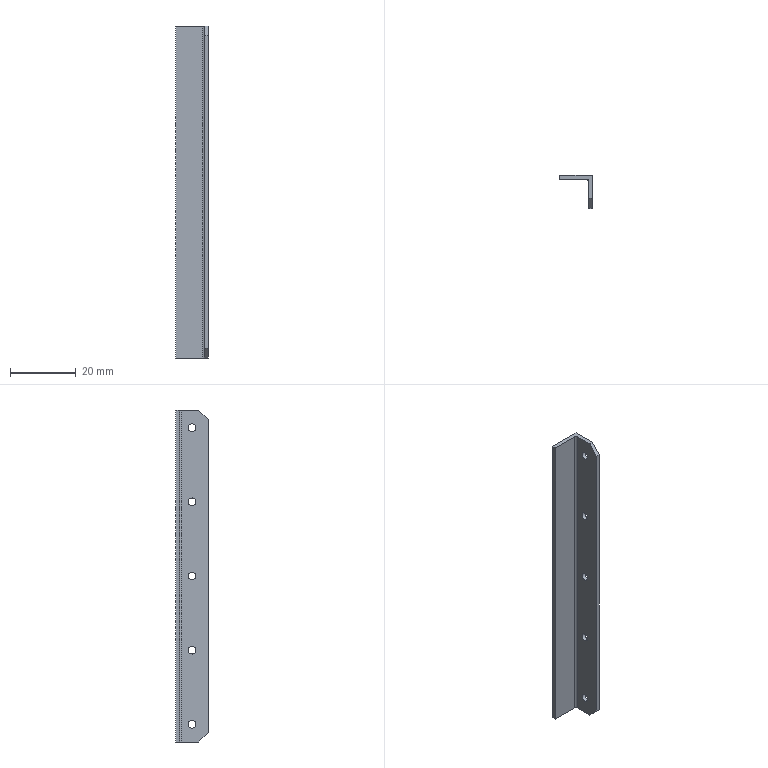Part | SolidWorks | features BaseBody 1 | 1 solid | 21 faces | box 10 x 10 x 100.8 mm | volume 2242 mm3 | cylinder 11 | plane 10 | commonest cylinder face diameters 2.4 x10 1 x1
STEP:
#1=CARTESIAN_POINT('',(-1.2,-5.,-74.1));
#2=VERTEX_POINT('',#1);
#3=CARTESIAN_POINT('',(-1.2,-5.,-71.7));
#4=VERTEX_POINT('',#3);
#5=CARTESIAN_POINT('',(-1.2,-5.,-72.9));
#6=DIRECTION('',(-1.,0.,0.));
#7=DIRECTION('',(0.,0.,-1.));
#8=AXIS2_PLACEMENT_3D('',#5,#6,#7);
#9=CIRCLE('',#8,1.2);
#10=EDGE_CURVE('',#2,#4,#9,.T.);
#11=ORIENTED_EDGE('',*,*,#10,.T.);
#12=CARTESIAN_POINT('',(0.,-5.,-71.7));
#13=VERTEX_POINT('',#12);
#14=CARTESIAN_POINT('',(-1.2,-5.,-71.7));
#15=DIRECTION('',(1.,0.,0.));
#16=VECTOR('',#15,1000.);
#17=LINE('',#14,#16);
#18=EDGE_CURVE('',#4,#13,#17,.T.);
#19=ORIENTED_EDGE('',*,*,#18,.T.);
#20=CARTESIAN_POINT('',(0.,-5.,-74.1));
#21=VERTEX_POINT('',#20);
#22=CARTESIAN_POINT('',(0.,-5.,-72.9));
#23=DIRECTION('',(1.,0.,0.));
#24=DIRECTION('',(0.,0.,-1.));
#25=AXIS2_PLACEMENT_3D('',#22,#23,#24);
#26=CIRCLE('',#25,1.2);
#27=EDGE_CURVE('',#13,#21,#26,.T.);
#28=ORIENTED_EDGE('',*,*,#27,.T.);
#29=CARTESIAN_POINT('',(-1.2,-5.,-74.1));
#30=DIRECTION('',(1.,0.,0.));
#31=VECTOR('',#30,1000.);
#32=LINE('',#29,#31);
#33=EDGE_CURVE('',#2,#21,#32,.T.);
#34=ORIENTED_EDGE('',*,*,#33,.F.);
#35=EDGE_LOOP('',(#11,#19,#28,#34));
#36=FACE_OUTER_BOUND('',#35,.T.);
#37=CARTESIAN_POINT('',(-1.2,-5.,-72.9));
#38=DIRECTION('',(1.,0.,0.));
#39=DIRECTION('',(0.,0.,-1.));
#40=AXIS2_PLACEMENT_3D('',#37,#38,#39);
#41=CYLINDRICAL_SURFACE('',#40,1.2);
#42=ADVANCED_FACE('',(#36),#41,.F.);
#43=CARTESIAN_POINT('',(-1.2,-5.,-96.6));
#44=VERTEX_POINT('',#43);
#45=CARTESIAN_POINT('',(-1.2,-5.,-94.2));
#46=VERTEX_POINT('',#45);
#47=CARTESIAN_POINT('',(-1.2,-5.,-95.4));
#48=DIRECTION('',(-1.,0.,0.));
#49=DIRECTION('',(0.,0.,-1.));
#50=AXIS2_PLACEMENT_3D('',#47,#48,#49);
#51=CIRCLE('',#50,1.2);
#52=EDGE_CURVE('',#44,#46,#51,.T.);
#53=ORIENTED_EDGE('',*,*,#52,.T.);
#54=CARTESIAN_POINT('',(0.,-5.,-94.2));
#55=VERTEX_POINT('',#54);
#56=CARTESIAN_POINT('',(-1.2,-5.,-94.2));
#57=DIRECTION('',(1.,0.,0.));
#58=VECTOR('',#57,1000.);
#59=LINE('',#56,#58);
#60=EDGE_CURVE('',#46,#55,#59,.T.);
#61=ORIENTED_EDGE('',*,*,#60,.T.);
#62=CARTESIAN_POINT('',(0.,-5.,-96.6));
#63=VERTEX_POINT('',#62);
#64=CARTESIAN_POINT('',(0.,-5.,-95.4));
#65=DIRECTION('',(1.,0.,0.));
#66=DIRECTION('',(0.,0.,-1.));
#67=AXIS2_PLACEMENT_3D('',#64,#65,#66);
#68=CIRCLE('',#67,1.2);
#69=EDGE_CURVE('',#55,#63,#68,.T.);
#70=ORIENTED_EDGE('',*,*,#69,.T.);
#71=CARTESIAN_POINT('',(-1.2,-5.,-96.6));
#72=DIRECTION('',(1.,0.,0.));
#73=VECTOR('',#72,1000.);
#74=LINE('',#71,#73);
#75=EDGE_CURVE('',#44,#63,#74,.T.);
#76=ORIENTED_EDGE('',*,*,#75,.F.);
#77=EDGE_LOOP('',(#53,#61,#70,#76));
#78=FACE_OUTER_BOUND('',#77,.T.);
#79=CARTESIAN_POINT('',(-1.2,-5.,-95.4));
#80=DIRECTION('',(1.,0.,0.));
#81=DIRECTION('',(0.,0.,-1.));
#82=AXIS2_PLACEMENT_3D('',#79,#80,#81);
#83=CYLINDRICAL_SURFACE('',#82,1.2);
#84=ADVANCED_FACE('',(#78),#83,.F.);
#85=CARTESIAN_POINT('',(-1.2,-5.,-6.6));
#86=VERTEX_POINT('',#85);
#87=CARTESIAN_POINT('',(-1.2,-5.,-4.2));
#88=VERTEX_POINT('',#87);
#89=CARTESIAN_POINT('',(-1.2,-5.,-5.4));
#90=DIRECTION('',(-1.,0.,0.));
#91=DIRECTION('',(0.,0.,-1.));
#92=AXIS2_PLACEMENT_3D('',#89,#90,#91);
#93=CIRCLE('',#92,1.2);
#94=EDGE_CURVE('',#86,#88,#93,.T.);
#95=ORIENTED_EDGE('',*,*,#94,.T.);
#96=CARTESIAN_POINT('',(0.,-5.,-4.2));
#97=VERTEX_POINT('',#96);
#98=CARTESIAN_POINT('',(-1.2,-5.,-4.2));
#99=DIRECTION('',(1.,0.,0.));
#100=VECTOR('',#99,1000.);
#101=LINE('',#98,#100);
#102=EDGE_CURVE('',#88,#97,#101,.T.);
#103=ORIENTED_EDGE('',*,*,#102,.T.);
#104=CARTESIAN_POINT('',(0.,-5.,-6.6));
#105=VERTEX_POINT('',#104);
#106=CARTESIAN_POINT('',(0.,-5.,-5.4));
#107=DIRECTION('',(1.,0.,0.));
#108=DIRECTION('',(0.,0.,-1.));
#109=AXIS2_PLACEMENT_3D('',#106,#107,#108);
#110=CIRCLE('',#109,1.2);
#111=EDGE_CURVE('',#97,#105,#110,.T.);
#112=ORIENTED_EDGE('',*,*,#111,.T.);
#113=CARTESIAN_POINT('',(-1.2,-5.,-6.6));
#114=DIRECTION('',(1.,0.,0.));
#115=VECTOR('',#114,1000.);
#116=LINE('',#113,#115);
#117=EDGE_CURVE('',#86,#105,#116,.T.);
#118=ORIENTED_EDGE('',*,*,#117,.F.);
#119=EDGE_LOOP('',(#95,#103,#112,#118));
#120=FACE_OUTER_BOUND('',#119,.T.);
#121=CARTESIAN_POINT('',(-1.2,-5.,-5.4));
#122=DIRECTION('',(1.,0.,0.));
#123=DIRECTION('',(0.,0.,-1.));
#124=AXIS2_PLACEMENT_3D('',#121,#122,#123);
#125=CYLINDRICAL_SURFACE('',#124,1.2);
#126=ADVANCED_FACE('',(#120),#125,.F.);
#127=CARTESIAN_POINT('',(-1.2,-5.,-51.6));
#128=VERTEX_POINT('',#127);
#129=CARTESIAN_POINT('',(-1.2,-5.,-49.2));
#130=VERTEX_POINT('',#129);
#131=CARTESIAN_POINT('',(-1.2,-5.,-50.4));
#132=DIRECTION('',(-1.,0.,0.));
#133=DIRECTION('',(0.,0.,-1.));
#134=AXIS2_PLACEMENT_3D('',#131,#132,#133);
#135=CIRCLE('',#134,1.2);
#136=EDGE_CURVE('',#128,#130,#135,.T.);
#137=ORIENTED_EDGE('',*,*,#136,.T.);
#138=CARTESIAN_POINT('',(0.,-5.,-49.2));
#139=VERTEX_POINT('',#138);
#140=CARTESIAN_POINT('',(-1.2,-5.,-49.2));
#141=DIRECTION('',(1.,0.,0.));
#142=VECTOR('',#141,1000.);
#143=LINE('',#140,#142);
#144=EDGE_CURVE('',#130,#139,#143,.T.);
#145=ORIENTED_EDGE('',*,*,#144,.T.);
#146=CARTESIAN_POINT('',(0.,-5.,-51.6));
#147=VERTEX_POINT('',#146);
#148=CARTESIAN_POINT('',(0.,-5.,-50.4));
#149=DIRECTION('',(1.,0.,0.));
#150=DIRECTION('',(0.,0.,-1.));
#151=AXIS2_PLACEMENT_3D('',#148,#149,#150);
#152=CIRCLE('',#151,1.2);
#153=EDGE_CURVE('',#139,#147,#152,.T.);
#154=ORIENTED_EDGE('',*,*,#153,.T.);
#155=CARTESIAN_POINT('',(-1.2,-5.,-51.6));
#156=DIRECTION('',(1.,0.,0.));
#157=VECTOR('',#156,1000.);
#158=LINE('',#155,#157);
#159=EDGE_CURVE('',#128,#147,#158,.T.);
#160=ORIENTED_EDGE('',*,*,#159,.F.);
#161=EDGE_LOOP('',(#137,#145,#154,#160));
#162=FACE_OUTER_BOUND('',#161,.T.);
#163=CARTESIAN_POINT('',(-1.2,-5.,-50.4));
#164=DIRECTION('',(1.,0.,0.));
#165=DIRECTION('',(0.,0.,-1.));
#166=AXIS2_PLACEMENT_3D('',#163,#164,#165);
#167=CYLINDRICAL_SURFACE('',#166,1.2);
#168=ADVANCED_FACE('',(#162),#167,.F.);
#169=CARTESIAN_POINT('',(-1.2,-5.,-29.1));
#170=VERTEX_POINT('',#169);
#171=CARTESIAN_POINT('',(-1.2,-5.,-26.7));
#172=VERTEX_POINT('',#171);
#173=CARTESIAN_POINT('',(-1.2,-5.,-27.9));
#174=DIRECTION('',(-1.,0.,0.));
#175=DIRECTION('',(0.,0.,-1.));
#176=AXIS2_PLACEMENT_3D('',#173,#174,#175);
#177=CIRCLE('',#176,1.2);
#178=EDGE_CURVE('',#170,#172,#177,.T.);
#179=ORIENTED_EDGE('',*,*,#178,.T.);
#180=CARTESIAN_POINT('',(0.,-5.,-26.7));
#181=VERTEX_POINT('',#180);
#182=CARTESIAN_POINT('',(-1.2,-5.,-26.7));
#183=DIRECTION('',(1.,0.,0.));
#184=VECTOR('',#183,1000.);
#185=LINE('',#182,#184);
#186=EDGE_CURVE('',#172,#181,#185,.T.);
#187=ORIENTED_EDGE('',*,*,#186,.T.);
#188=CARTESIAN_POINT('',(0.,-5.,-29.1));
#189=VERTEX_POINT('',#188);
#190=CARTESIAN_POINT('',(0.,-5.,-27.9));
#191=DIRECTION('',(1.,0.,0.));
#192=DIRECTION('',(0.,0.,-1.));
#193=AXIS2_PLACEMENT_3D('',#190,#191,#192);
#194=CIRCLE('',#193,1.2);
#195=EDGE_CURVE('',#181,#189,#194,.T.);
#196=ORIENTED_EDGE('',*,*,#195,.T.);
#197=CARTESIAN_POINT('',(-1.2,-5.,-29.1));
#198=DIRECTION('',(1.,0.,0.));
#199=VECTOR('',#198,1000.);
#200=LINE('',#197,#199);
#201=EDGE_CURVE('',#170,#189,#200,.T.);
#202=ORIENTED_EDGE('',*,*,#201,.F.);
#203=EDGE_LOOP('',(#179,#187,#196,#202));
#204=FACE_OUTER_BOUND('',#203,.T.);
#205=CARTESIAN_POINT('',(-1.2,-5.,-27.9));
#206=DIRECTION('',(1.,0.,0.));
#207=DIRECTION('',(0.,0.,-1.));
#208=AXIS2_PLACEMENT_3D('',#205,#206,#207);
#209=CYLINDRICAL_SURFACE('',#208,1.2);
#210=ADVANCED_FACE('',(#204),#209,.F.);
#211=ORIENTED_EDGE('',*,*,#18,.F.);
#212=CARTESIAN_POINT('',(-1.2,-5.,-72.9));
#213=DIRECTION('',(-1.,0.,0.));
#214=DIRECTION('',(0.,0.,-1.));
#215=AXIS2_PLACEMENT_3D('',#212,#213,#214);
#216=CIRCLE('',#215,1.2);
#217=EDGE_CURVE('',#4,#2,#216,.T.);
#218=ORIENTED_EDGE('',*,*,#217,.T.);
#219=ORIENTED_EDGE('',*,*,#33,.T.);
#220=CARTESIAN_POINT('',(0.,-5.,-72.9));
#221=DIRECTION('',(1.,0.,0.));
#222=DIRECTION('',(0.,0.,-1.));
#223=AXIS2_PLACEMENT_3D('',#220,#221,#222);
#224=CIRCLE('',#223,1.2);
#225=EDGE_CURVE('',#21,#13,#224,.T.);
#226=ORIENTED_EDGE('',*,*,#225,.T.);
#227=EDGE_LOOP('',(#211,#218,#219,#226));
#228=FACE_OUTER_BOUND('',#227,.T.);
#229=CARTESIAN_POINT('',(-1.2,-5.,-72.9));
#230=DIRECTION('',(1.,0.,0.));
#231=DIRECTION('',(0.,0.,-1.));
#232=AXIS2_PLACEMENT_3D('',#229,#230,#231);
#233=CYLINDRICAL_SURFACE('',#232,1.2);
#234=ADVANCED_FACE('',(#228),#233,.F.);
#235=CARTESIAN_POINT('',(0.,-5.,-95.4));
#236=DIRECTION('',(1.,0.,0.));
#237=DIRECTION('',(0.,0.,-1.));
#238=AXIS2_PLACEMENT_3D('',#235,#236,#237);
#239=CIRCLE('',#238,1.2);
#240=EDGE_CURVE('',#63,#55,#239,.T.);
#241=ORIENTED_EDGE('',*,*,#240,.F.);
#242=ORIENTED_EDGE('',*,*,#69,.F.);
#243=EDGE_LOOP('',(#241,#242));
#244=FACE_BOUND('',#243,.T.);
#245=CARTESIAN_POINT('',(0.,-5.,-5.4));
#246=DIRECTION('',(1.,0.,0.));
#247=DIRECTION('',(0.,0.,-1.));
#248=AXIS2_PLACEMENT_3D('',#245,#246,#247);
#249=CIRCLE('',#248,1.2);
#250=EDGE_CURVE('',#105,#97,#249,.T.);
#251=ORIENTED_EDGE('',*,*,#250,.F.);
#252=ORIENTED_EDGE('',*,*,#111,.F.);
#253=EDGE_LOOP('',(#251,#252));
#254=FACE_BOUND('',#253,.T.);
#255=CARTESIAN_POINT('',(0.,-5.,-50.4));
#256=DIRECTION('',(1.,0.,0.));
#257=DIRECTION('',(0.,0.,-1.));
#258=AXIS2_PLACEMENT_3D('',#255,#256,#257);
#259=CIRCLE('',#258,1.2);
#260=EDGE_CURVE('',#147,#139,#259,.T.);
#261=ORIENTED_EDGE('',*,*,#260,.F.);
#262=ORIENTED_EDGE('',*,*,#153,.F.);
#263=EDGE_LOOP('',(#261,#262));
#264=FACE_BOUND('',#263,.T.);
#265=CARTESIAN_POINT('',(0.,-5.,-27.9));
#266=DIRECTION('',(1.,0.,0.));
#267=DIRECTION('',(0.,0.,-1.));
#268=AXIS2_PLACEMENT_3D('',#265,#266,#267);
#269=CIRCLE('',#268,1.2);
#270=EDGE_CURVE('',#189,#181,#269,.T.);
#271=ORIENTED_EDGE('',*,*,#270,.F.);
#272=ORIENTED_EDGE('',*,*,#195,.F.);
#273=EDGE_LOOP('',(#271,#272));
#274=FACE_BOUND('',#273,.T.);
#275=ORIENTED_EDGE('',*,*,#225,.F.);
#276=ORIENTED_EDGE('',*,*,#27,.F.);
#277=EDGE_LOOP('',(#275,#276));
#278=FACE_BOUND('',#277,.T.);
#279=CARTESIAN_POINT('',(0.,0.,0.));
#280=VERTEX_POINT('',#279);
#281=CARTESIAN_POINT('',(0.,0.,-100.8));
#282=VERTEX_POINT('',#281);
#283=CARTESIAN_POINT('',(0.,0.,-50.4));
#284=DIRECTION('',(0.,0.,-1.));
#285=VECTOR('',#284,1000.);
#286=LINE('',#283,#285);
#287=EDGE_CURVE('',#280,#282,#286,.T.);
#288=ORIENTED_EDGE('',*,*,#287,.F.);
#289=CARTESIAN_POINT('',(0.,-7.,0.));
#290=VERTEX_POINT('',#289);
#291=CARTESIAN_POINT('',(0.,-5.,0.));
#292=DIRECTION('',(0.,1.,0.));
#293=VECTOR('',#292,1000.);
#294=LINE('',#291,#293);
#295=EDGE_CURVE('',#290,#280,#294,.T.);
#296=ORIENTED_EDGE('',*,*,#295,.F.);
#297=CARTESIAN_POINT('',(0.,-10.,-3.));
#298=VERTEX_POINT('',#297);
#299=CARTESIAN_POINT('',(0.,-10.,-3.));
#300=DIRECTION('',(0.,0.7071,0.7071));
#301=VECTOR('',#300,1000.);
#302=LINE('',#299,#301);
#303=EDGE_CURVE('',#298,#290,#302,.T.);
#304=ORIENTED_EDGE('',*,*,#303,.F.);
#305=CARTESIAN_POINT('',(0.,-10.,-97.8));
#306=VERTEX_POINT('',#305);
#307=CARTESIAN_POINT('',(0.,-10.,-50.4));
#308=DIRECTION('',(0.,0.,1.));
#309=VECTOR('',#308,1000.);
#310=LINE('',#307,#309);
#311=EDGE_CURVE('',#306,#298,#310,.T.);
#312=ORIENTED_EDGE('',*,*,#311,.F.);
#313=CARTESIAN_POINT('',(0.,-7.,-100.8));
#314=VERTEX_POINT('',#313);
#315=CARTESIAN_POINT('',(0.,-10.,-97.8));
#316=DIRECTION('',(0.,-0.7071,0.7071));
#317=VECTOR('',#316,1000.);
#318=LINE('',#315,#317);
#319=EDGE_CURVE('',#314,#306,#318,.T.);
#320=ORIENTED_EDGE('',*,*,#319,.F.);
#321=CARTESIAN_POINT('',(0.,-5.,-100.8));
#322=DIRECTION('',(0.,-1.,0.));
#323=VECTOR('',#322,1000.);
#324=LINE('',#321,#323);
#325=EDGE_CURVE('',#282,#314,#324,.T.);
#326=ORIENTED_EDGE('',*,*,#325,.F.);
#327=EDGE_LOOP('',(#288,#296,#304,#312,#320,#326));
#328=FACE_OUTER_BOUND('',#327,.T.);
#329=CARTESIAN_POINT('',(0.,0.,-100.8));
#330=DIRECTION('',(-1.,0.,0.));
#331=DIRECTION('',(0.,-1.,0.));
#332=AXIS2_PLACEMENT_3D('',#329,#330,#331);
#333=PLANE('',#332);
#334=ADVANCED_FACE('',(#244,#254,#264,#274,#278,#328),#333,.F.);
#335=ORIENTED_EDGE('',*,*,#52,.F.);
#336=CARTESIAN_POINT('',(-1.2,-5.,-95.4));
#337=DIRECTION('',(-1.,0.,0.));
#338=DIRECTION('',(0.,0.,-1.));
#339=AXIS2_PLACEMENT_3D('',#336,#337,#338);
#340=CIRCLE('',#339,1.2);
#341=EDGE_CURVE('',#46,#44,#340,.T.);
#342=ORIENTED_EDGE('',*,*,#341,.F.);
#343=EDGE_LOOP('',(#335,#342));
#344=FACE_BOUND('',#343,.T.);
#345=ORIENTED_EDGE('',*,*,#94,.F.);
#346=CARTESIAN_POINT('',(-1.2,-5.,-5.4));
#347=DIRECTION('',(-1.,0.,0.));
#348=DIRECTION('',(0.,0.,-1.));
#349=AXIS2_PLACEMENT_3D('',#346,#347,#348);
#350=CIRCLE('',#349,1.2);
#351=EDGE_CURVE('',#88,#86,#350,.T.);
#352=ORIENTED_EDGE('',*,*,#351,.F.);
#353=EDGE_LOOP('',(#345,#352));
#354=FACE_BOUND('',#353,.T.);
#355=ORIENTED_EDGE('',*,*,#136,.F.);
#356=CARTESIAN_POINT('',(-1.2,-5.,-50.4));
#357=DIRECTION('',(-1.,0.,0.));
#358=DIRECTION('',(0.,0.,-1.));
#359=AXIS2_PLACEMENT_3D('',#356,#357,#358);
#360=CIRCLE('',#359,1.2);
#361=EDGE_CURVE('',#130,#128,#360,.T.);
#362=ORIENTED_EDGE('',*,*,#361,.F.);
#363=EDGE_LOOP('',(#355,#362));
#364=FACE_BOUND('',#363,.T.);
#365=ORIENTED_EDGE('',*,*,#178,.F.);
#366=CARTESIAN_POINT('',(-1.2,-5.,-27.9));
#367=DIRECTION('',(-1.,0.,0.));
#368=DIRECTION('',(0.,0.,-1.));
#369=AXIS2_PLACEMENT_3D('',#366,#367,#368);
#370=CIRCLE('',#369,1.2);
#371=EDGE_CURVE('',#172,#170,#370,.T.);
#372=ORIENTED_EDGE('',*,*,#371,.F.);
#373=EDGE_LOOP('',(#365,#372));
#374=FACE_BOUND('',#373,.T.);
#375=ORIENTED_EDGE('',*,*,#10,.F.);
#376=ORIENTED_EDGE('',*,*,#217,.F.);
#377=EDGE_LOOP('',(#375,#376));
#378=FACE_BOUND('',#377,.T.);
#379=CARTESIAN_POINT('',(-1.2,-7.,0.));
#380=VERTEX_POINT('',#379);
#381=CARTESIAN_POINT('',(-1.2,-10.,-3.));
#382=VERTEX_POINT('',#381);
#383=CARTESIAN_POINT('',(-1.2,-10.,-3.));
#384=DIRECTION('',(0.,-0.7071,-0.7071));
#385=VECTOR('',#384,1000.);
#386=LINE('',#383,#385);
#387=EDGE_CURVE('',#380,#382,#386,.T.);
#388=ORIENTED_EDGE('',*,*,#387,.F.);
#389=CARTESIAN_POINT('',(-1.2,-1.7,0.));
#390=VERTEX_POINT('',#389);
#391=CARTESIAN_POINT('',(-1.2,-5.85,0.));
#392=DIRECTION('',(0.,-1.,0.));
#393=VECTOR('',#392,1000.);
#394=LINE('',#391,#393);
#395=EDGE_CURVE('',#390,#380,#394,.T.);
#396=ORIENTED_EDGE('',*,*,#395,.F.);
#397=CARTESIAN_POINT('',(-1.2,-1.7,-100.8));
#398=VERTEX_POINT('',#397);
#399=CARTESIAN_POINT('',(-1.2,-1.7,-50.4));
#400=DIRECTION('',(0.,0.,1.));
#401=VECTOR('',#400,1000.);
#402=LINE('',#399,#401);
#403=EDGE_CURVE('',#398,#390,#402,.T.);
#404=ORIENTED_EDGE('',*,*,#403,.F.);
#405=CARTESIAN_POINT('',(-1.2,-7.,-100.8));
#406=VERTEX_POINT('',#405);
#407=CARTESIAN_POINT('',(-1.2,-5.85,-100.8));
#408=DIRECTION('',(0.,1.,0.));
#409=VECTOR('',#408,1000.);
#410=LINE('',#407,#409);
#411=EDGE_CURVE('',#406,#398,#410,.T.);
#412=ORIENTED_EDGE('',*,*,#411,.F.);
#413=CARTESIAN_POINT('',(-1.2,-10.,-97.8));
#414=VERTEX_POINT('',#413);
#415=CARTESIAN_POINT('',(-1.2,-10.,-97.8));
#416=DIRECTION('',(0.,0.7071,-0.7071));
#417=VECTOR('',#416,1000.);
#418=LINE('',#415,#417);
#419=EDGE_CURVE('',#414,#406,#418,.T.);
#420=ORIENTED_EDGE('',*,*,#419,.F.);
#421=CARTESIAN_POINT('',(-1.2,-10.,-50.4));
#422=DIRECTION('',(0.,0.,-1.));
#423=VECTOR('',#422,1000.);
#424=LINE('',#421,#423);
#425=EDGE_CURVE('',#382,#414,#424,.T.);
#426=ORIENTED_EDGE('',*,*,#425,.F.);
#427=EDGE_LOOP('',(#388,#396,#404,#412,#420,#426));
#428=FACE_OUTER_BOUND('',#427,.T.);
#429=CARTESIAN_POINT('',(-1.2,-10.,-100.8));
#430=DIRECTION('',(1.,0.,0.));
#431=DIRECTION('',(0.,1.,0.));
#432=AXIS2_PLACEMENT_3D('',#429,#430,#431);
#433=PLANE('',#432);
#434=ADVANCED_FACE('',(#344,#354,#364,#374,#378,#428),#433,.F.);
#435=ORIENTED_EDGE('',*,*,#60,.F.);
#436=ORIENTED_EDGE('',*,*,#341,.T.);
#437=ORIENTED_EDGE('',*,*,#75,.T.);
#438=ORIENTED_EDGE('',*,*,#240,.T.);
#439=EDGE_LOOP('',(#435,#436,#437,#438));
#440=FACE_OUTER_BOUND('',#439,.T.);
#441=CARTESIAN_POINT('',(-1.2,-5.,-95.4));
#442=DIRECTION('',(1.,0.,0.));
#443=DIRECTION('',(0.,0.,-1.));
#444=AXIS2_PLACEMENT_3D('',#441,#442,#443);
#445=CYLINDRICAL_SURFACE('',#444,1.2);
#446=ADVANCED_FACE('',(#440),#445,.F.);
#447=ORIENTED_EDGE('',*,*,#102,.F.);
#448=ORIENTED_EDGE('',*,*,#351,.T.);
#449=ORIENTED_EDGE('',*,*,#117,.T.);
#450=ORIENTED_EDGE('',*,*,#250,.T.);
#451=EDGE_LOOP('',(#447,#448,#449,#450));
#452=FACE_OUTER_BOUND('',#451,.T.);
#453=CARTESIAN_POINT('',(-1.2,-5.,-5.4));
#454=DIRECTION('',(1.,0.,0.));
#455=DIRECTION('',(0.,0.,-1.));
#456=AXIS2_PLACEMENT_3D('',#453,#454,#455);
#457=CYLINDRICAL_SURFACE('',#456,1.2);
#458=ADVANCED_FACE('',(#452),#457,.F.);
#459=ORIENTED_EDGE('',*,*,#144,.F.);
#460=ORIENTED_EDGE('',*,*,#361,.T.);
#461=ORIENTED_EDGE('',*,*,#159,.T.);
#462=ORIENTED_EDGE('',*,*,#260,.T.);
#463=EDGE_LOOP('',(#459,#460,#461,#462));
#464=FACE_OUTER_BOUND('',#463,.T.);
#465=CARTESIAN_POINT('',(-1.2,-5.,-50.4));
#466=DIRECTION('',(1.,0.,0.));
#467=DIRECTION('',(0.,0.,-1.));
#468=AXIS2_PLACEMENT_3D('',#465,#466,#467);
#469=CYLINDRICAL_SURFACE('',#468,1.2);
#470=ADVANCED_FACE('',(#464),#469,.F.);
#471=ORIENTED_EDGE('',*,*,#186,.F.);
#472=ORIENTED_EDGE('',*,*,#371,.T.);
#473=ORIENTED_EDGE('',*,*,#201,.T.);
#474=ORIENTED_EDGE('',*,*,#270,.T.);
#475=EDGE_LOOP('',(#471,#472,#473,#474));
#476=FACE_OUTER_BOUND('',#475,.T.);
#477=CARTESIAN_POINT('',(-1.2,-5.,-27.9));
#478=DIRECTION('',(1.,0.,0.));
#479=DIRECTION('',(0.,0.,-1.));
#480=AXIS2_PLACEMENT_3D('',#477,#478,#479);
#481=CYLINDRICAL_SURFACE('',#480,1.2);
#482=ADVANCED_FACE('',(#476),#481,.F.);
#483=CARTESIAN_POINT('',(-1.7,-1.2,-100.8));
#484=VERTEX_POINT('',#483);
#485=CARTESIAN_POINT('',(-1.7,-1.7,-100.8));
#486=DIRECTION('',(0.,0.,-1.));
#487=DIRECTION('',(1.,0.,0.));
#488=AXIS2_PLACEMENT_3D('',#485,#486,#487);
#489=CIRCLE('',#488,0.5);
#490=EDGE_CURVE('',#484,#398,#489,.T.);
#491=ORIENTED_EDGE('',*,*,#490,.F.);
#492=CARTESIAN_POINT('',(-10.,-1.2,-100.8));
#493=VERTEX_POINT('',#492);
#494=CARTESIAN_POINT('',(-5.,-1.2,-100.8));
#495=DIRECTION('',(1.,0.,0.));
#496=VECTOR('',#495,1000.);
#497=LINE('',#494,#496);
#498=EDGE_CURVE('',#493,#484,#497,.T.);
#499=ORIENTED_EDGE('',*,*,#498,.F.);
#500=CARTESIAN_POINT('',(-10.,0.,-100.8));
#501=VERTEX_POINT('',#500);
#502=CARTESIAN_POINT('',(-10.,-0.6,-100.8));
#503=DIRECTION('',(0.,1.,0.));
#504=VECTOR('',#503,1000.);
#505=LINE('',#502,#504);
#506=EDGE_CURVE('',#493,#501,#505,.T.);
#507=ORIENTED_EDGE('',*,*,#506,.T.);
#508=CARTESIAN_POINT('',(-5.,0.,-100.8));
#509=DIRECTION('',(-1.,0.,0.));
#510=VECTOR('',#509,1000.);
#511=LINE('',#508,#510);
#512=EDGE_CURVE('',#282,#501,#511,.T.);
#513=ORIENTED_EDGE('',*,*,#512,.F.);
#514=ORIENTED_EDGE('',*,*,#325,.T.);
#515=CARTESIAN_POINT('',(-5.,-7.,-100.8));
#516=DIRECTION('',(1.,0.,0.));
#517=VECTOR('',#516,1000.);
#518=LINE('',#515,#517);
#519=EDGE_CURVE('',#406,#314,#518,.T.);
#520=ORIENTED_EDGE('',*,*,#519,.F.);
#521=ORIENTED_EDGE('',*,*,#411,.T.);
#522=EDGE_LOOP('',(#491,#499,#507,#513,#514,#520,#521));
#523=FACE_OUTER_BOUND('',#522,.T.);
#524=CARTESIAN_POINT('',(0.,0.,-100.8));
#525=DIRECTION('',(0.,0.,1.));
#526=DIRECTION('',(-1.,0.,0.));
#527=AXIS2_PLACEMENT_3D('',#524,#525,#526);
#528=PLANE('',#527);
#529=ADVANCED_FACE('',(#523),#528,.F.);
#530=ORIENTED_EDGE('',*,*,#287,.T.);
#531=ORIENTED_EDGE('',*,*,#512,.T.);
#532=CARTESIAN_POINT('',(-10.,0.,0.));
#533=VERTEX_POINT('',#532);
#534=CARTESIAN_POINT('',(-10.,0.,-50.4));
#535=DIRECTION('',(0.,0.,-1.));
#536=VECTOR('',#535,1000.);
#537=LINE('',#534,#536);
#538=EDGE_CURVE('',#533,#501,#537,.T.);
#539=ORIENTED_EDGE('',*,*,#538,.F.);
#540=CARTESIAN_POINT('',(-5.,0.,0.));
#541=DIRECTION('',(-1.,0.,0.));
#542=VECTOR('',#541,1000.);
#543=LINE('',#540,#542);
#544=EDGE_CURVE('',#280,#533,#543,.T.);
#545=ORIENTED_EDGE('',*,*,#544,.F.);
#546=EDGE_LOOP('',(#530,#531,#539,#545));
#547=FACE_OUTER_BOUND('',#546,.T.);
#548=CARTESIAN_POINT('',(-10.,0.,-100.8));
#549=DIRECTION('',(0.,-1.,0.));
#550=DIRECTION('',(1.,0.,0.));
#551=AXIS2_PLACEMENT_3D('',#548,#549,#550);
#552=PLANE('',#551);
#553=ADVANCED_FACE('',(#547),#552,.F.);
#554=ORIENTED_EDGE('',*,*,#395,.T.);
#555=CARTESIAN_POINT('',(-5.,-7.,0.));
#556=DIRECTION('',(1.,0.,0.));
#557=VECTOR('',#556,1000.);
#558=LINE('',#555,#557);
#559=EDGE_CURVE('',#380,#290,#558,.T.);
#560=ORIENTED_EDGE('',*,*,#559,.T.);
#561=ORIENTED_EDGE('',*,*,#295,.T.);
#562=ORIENTED_EDGE('',*,*,#544,.T.);
#563=CARTESIAN_POINT('',(-10.,-1.2,0.));
#564=VERTEX_POINT('',#563);
#565=CARTESIAN_POINT('',(-10.,-3.5,0.));
#566=DIRECTION('',(0.,-1.,0.));
#567=VECTOR('',#566,1000.);
#568=LINE('',#565,#567);
#569=EDGE_CURVE('',#533,#564,#568,.T.);
#570=ORIENTED_EDGE('',*,*,#569,.T.);
#571=CARTESIAN_POINT('',(-1.7,-1.2,0.));
#572=VERTEX_POINT('',#571);
#573=CARTESIAN_POINT('',(-5.,-1.2,0.));
#574=DIRECTION('',(1.,0.,0.));
#575=VECTOR('',#574,1000.);
#576=LINE('',#573,#575);
#577=EDGE_CURVE('',#564,#572,#576,.T.);
#578=ORIENTED_EDGE('',*,*,#577,.T.);
#579=CARTESIAN_POINT('',(-1.7,-1.7,0.));
#580=DIRECTION('',(0.,0.,-1.));
#581=DIRECTION('',(1.,0.,0.));
#582=AXIS2_PLACEMENT_3D('',#579,#580,#581);
#583=CIRCLE('',#582,0.5);
#584=EDGE_CURVE('',#572,#390,#583,.T.);
#585=ORIENTED_EDGE('',*,*,#584,.T.);
#586=EDGE_LOOP('',(#554,#560,#561,#562,#570,#578,#585));
#587=FACE_OUTER_BOUND('',#586,.T.);
#588=CARTESIAN_POINT('',(0.,0.,0.));
#589=DIRECTION('',(0.,0.,1.));
#590=DIRECTION('',(-1.,0.,0.));
#591=AXIS2_PLACEMENT_3D('',#588,#589,#590);
#592=PLANE('',#591);
#593=ADVANCED_FACE('',(#587),#592,.T.);
#594=ORIENTED_EDGE('',*,*,#303,.T.);
#595=ORIENTED_EDGE('',*,*,#559,.F.);
#596=ORIENTED_EDGE('',*,*,#387,.T.);
#597=CARTESIAN_POINT('',(-0.6,-10.,-3.));
#598=DIRECTION('',(1.,0.,0.));
#599=VECTOR('',#598,1000.);
#600=LINE('',#597,#599);
#601=EDGE_CURVE('',#382,#298,#600,.T.);
#602=ORIENTED_EDGE('',*,*,#601,.T.);
#603=EDGE_LOOP('',(#594,#595,#596,#602));
#604=FACE_OUTER_BOUND('',#603,.T.);
#605=CARTESIAN_POINT('',(0.,-10.,-3.));
#606=DIRECTION('',(0.,-0.7071,0.7071));
#607=DIRECTION('',(0.,0.7071,0.7071));
#608=AXIS2_PLACEMENT_3D('',#605,#606,#607);
#609=PLANE('',#608);
#610=ADVANCED_FACE('',(#604),#609,.T.);
#611=ORIENTED_EDGE('',*,*,#601,.F.);
#612=ORIENTED_EDGE('',*,*,#425,.T.);
#613=CARTESIAN_POINT('',(-0.6,-10.,-97.8));
#614=DIRECTION('',(-1.,0.,0.));
#615=VECTOR('',#614,1000.);
#616=LINE('',#613,#615);
#617=EDGE_CURVE('',#306,#414,#616,.T.);
#618=ORIENTED_EDGE('',*,*,#617,.F.);
#619=ORIENTED_EDGE('',*,*,#311,.T.);
#620=EDGE_LOOP('',(#611,#612,#618,#619));
#621=FACE_OUTER_BOUND('',#620,.T.);
#622=CARTESIAN_POINT('',(0.,-10.,-3.));
#623=DIRECTION('',(0.,1.,0.));
#624=DIRECTION('',(0.,0.,-1.));
#625=AXIS2_PLACEMENT_3D('',#622,#623,#624);
#626=PLANE('',#625);
#627=ADVANCED_FACE('',(#621),#626,.F.);
#628=ORIENTED_EDGE('',*,*,#519,.T.);
#629=ORIENTED_EDGE('',*,*,#319,.T.);
#630=ORIENTED_EDGE('',*,*,#617,.T.);
#631=ORIENTED_EDGE('',*,*,#419,.T.);
#632=EDGE_LOOP('',(#628,#629,#630,#631));
#633=FACE_OUTER_BOUND('',#632,.T.);
#634=CARTESIAN_POINT('',(0.,-10.,-97.8));
#635=DIRECTION('',(0.,0.7071,0.7071));
#636=DIRECTION('',(0.,0.7071,-0.7071));
#637=AXIS2_PLACEMENT_3D('',#634,#635,#636);
#638=PLANE('',#637);
#639=ADVANCED_FACE('',(#633),#638,.F.);
#640=ORIENTED_EDGE('',*,*,#490,.T.);
#641=ORIENTED_EDGE('',*,*,#403,.T.);
#642=ORIENTED_EDGE('',*,*,#584,.F.);
#643=CARTESIAN_POINT('',(-1.7,-1.2,-50.4));
#644=DIRECTION('',(0.,0.,-1.));
#645=VECTOR('',#644,1000.);
#646=LINE('',#643,#645);
#647=EDGE_CURVE('',#572,#484,#646,.T.);
#648=ORIENTED_EDGE('',*,*,#647,.T.);
#649=EDGE_LOOP('',(#640,#641,#642,#648));
#650=FACE_OUTER_BOUND('',#649,.T.);
#651=CARTESIAN_POINT('',(-1.7,-1.7,-100.8));
#652=DIRECTION('',(0.,0.,1.));
#653=DIRECTION('',(1.,0.,0.));
#654=AXIS2_PLACEMENT_3D('',#651,#652,#653);
#655=CYLINDRICAL_SURFACE('',#654,0.5);
#656=ADVANCED_FACE('',(#650),#655,.F.);
#657=CARTESIAN_POINT('',(-10.,-1.2,-50.4));
#658=DIRECTION('',(0.,0.,1.));
#659=VECTOR('',#658,1000.);
#660=LINE('',#657,#659);
#661=EDGE_CURVE('',#493,#564,#660,.T.);
#662=ORIENTED_EDGE('',*,*,#661,.F.);
#663=ORIENTED_EDGE('',*,*,#498,.T.);
#664=ORIENTED_EDGE('',*,*,#647,.F.);
#665=ORIENTED_EDGE('',*,*,#577,.F.);
#666=EDGE_LOOP('',(#662,#663,#664,#665));
#667=FACE_OUTER_BOUND('',#666,.T.);
#668=CARTESIAN_POINT('',(-1.7,-1.2,-100.8));
#669=DIRECTION('',(0.,1.,0.));
#670=DIRECTION('',(-1.,0.,0.));
#671=AXIS2_PLACEMENT_3D('',#668,#669,#670);
#672=PLANE('',#671);
#673=ADVANCED_FACE('',(#667),#672,.F.);
#674=ORIENTED_EDGE('',*,*,#538,.T.);
#675=ORIENTED_EDGE('',*,*,#506,.F.);
#676=ORIENTED_EDGE('',*,*,#661,.T.);
#677=ORIENTED_EDGE('',*,*,#569,.F.);
#678=EDGE_LOOP('',(#674,#675,#676,#677));
#679=FACE_OUTER_BOUND('',#678,.T.);
#680=CARTESIAN_POINT('',(-10.,0.,-100.8));
#681=DIRECTION('',(1.,0.,0.));
#682=DIRECTION('',(0.,0.,1.));
#683=AXIS2_PLACEMENT_3D('',#680,#681,#682);
#684=PLANE('',#683);
#685=ADVANCED_FACE('',(#679),#684,.F.);
#686=CLOSED_SHELL('',(#42,#84,#126,#168,#210,#234,#334,#434,#446,#458,#470,#482,#529,#553,#593,#610,#627,#639,#656,#673,#685));
#687=MANIFOLD_SOLID_BREP('',#686);
#688=CARTESIAN_POINT('',(0.,0.,0.));
#689=DIRECTION('',(0.,0.,1.));
#690=DIRECTION('',(1.,0.,0.));
#691=AXIS2_PLACEMENT_3D('',#688,#689,#690);
#692=(LENGTH_UNIT()NAMED_UNIT(*)SI_UNIT(.MILLI.,.METRE.));
#693=UNCERTAINTY_MEASURE_WITH_UNIT(LENGTH_MEASURE(0.00001),#692,'','');
#694=(NAMED_UNIT(*)PLANE_ANGLE_UNIT()SI_UNIT($,.RADIAN.));
#695=(NAMED_UNIT(*)SI_UNIT($,.STERADIAN.)SOLID_ANGLE_UNIT());
#696=(GEOMETRIC_REPRESENTATION_CONTEXT(3)GLOBAL_UNCERTAINTY_ASSIGNED_CONTEXT((#693))GLOBAL_UNIT_ASSIGNED_CONTEXT((#692,#694,#695))REPRESENTATION_CONTEXT('',''));
#697=ADVANCED_BREP_SHAPE_REPRESENTATION('',(#687,#691),#696);